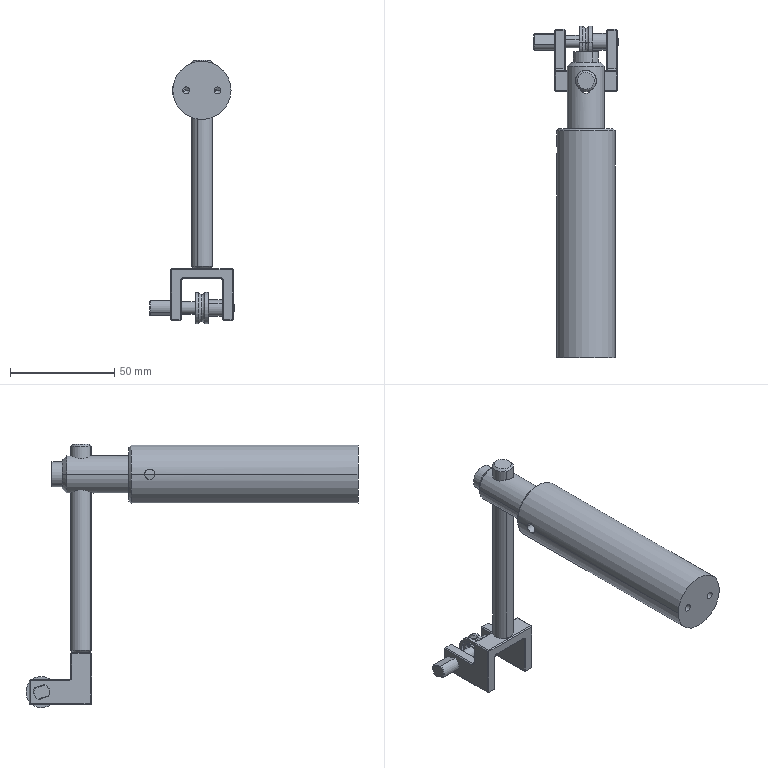Part | SolidWorks | 9 solids | 264 faces | box 40.5 x 159.5 x 126.5 mm | volume 84621 mm3 | plane 81 | cylinder 65 | cone 48 | torus 48 | sphere 22 | commonest cylinder face diameters 4 x8 3.3 x6 12 x6 2 x4 2.5 x4 6.667 x4